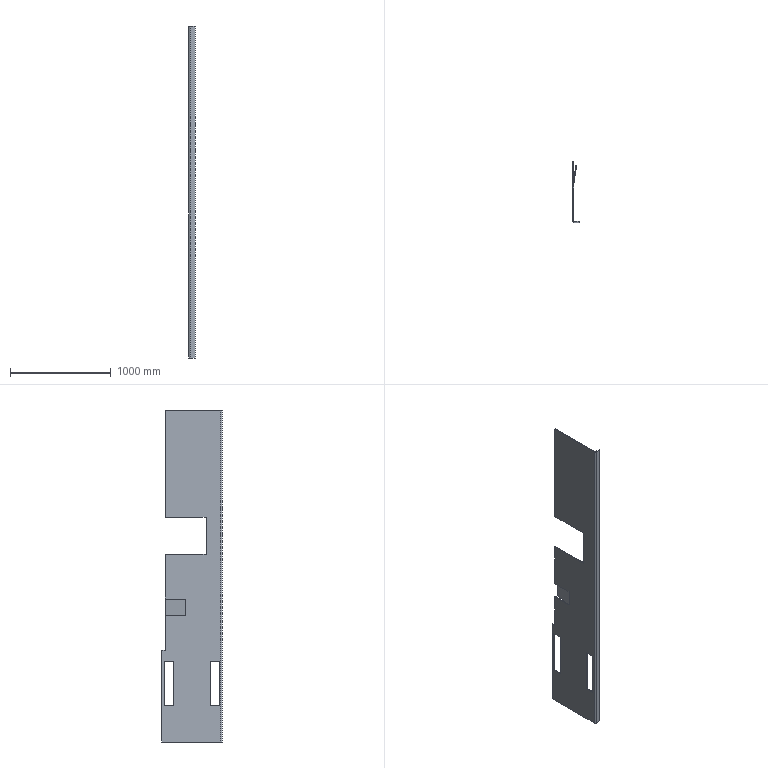Part | SolidWorks | features ICE 2, Extrusion 1, NetBlend 1 | 1 solid | 33 faces | box 65 x 605 x 3295 mm | volume 14782369 mm3 | plane 31 | cylinder 2 | commonest cylinder face diameters 16 x1 32 x1
STEP:
#1=CARTESIAN_POINT('',(0.,568.,909.));
#2=VERTEX_POINT('',#1);
#3=CARTESIAN_POINT('',(0.,568.,1259.));
#4=VERTEX_POINT('',#3);
#5=CARTESIAN_POINT('',(0.,568.,909.));
#6=DIRECTION('',(0.,0.,1.));
#7=VECTOR('',#6,1000.);
#8=LINE('',#5,#7);
#9=EDGE_CURVE('',#2,#4,#8,.T.);
#10=ORIENTED_EDGE('',*,*,#9,.T.);
#11=CARTESIAN_POINT('',(8.,568.,1259.));
#12=VERTEX_POINT('',#11);
#13=CARTESIAN_POINT('',(65.,568.,1259.));
#14=DIRECTION('',(-1.,0.,0.));
#15=VECTOR('',#14,1000.);
#16=LINE('',#13,#15);
#17=EDGE_CURVE('',#12,#4,#16,.T.);
#18=ORIENTED_EDGE('',*,*,#17,.F.);
#19=CARTESIAN_POINT('',(8.,568.,909.));
#20=VERTEX_POINT('',#19);
#21=CARTESIAN_POINT('',(8.,568.,3295.));
#22=DIRECTION('',(0.,0.,1.));
#23=VECTOR('',#22,1000.);
#24=LINE('',#21,#23);
#25=EDGE_CURVE('',#20,#12,#24,.T.);
#26=ORIENTED_EDGE('',*,*,#25,.F.);
#27=CARTESIAN_POINT('',(65.,568.,909.));
#28=DIRECTION('',(-1.,0.,0.));
#29=VECTOR('',#28,1000.);
#30=LINE('',#27,#29);
#31=EDGE_CURVE('',#20,#2,#30,.T.);
#32=ORIENTED_EDGE('',*,*,#31,.T.);
#33=EDGE_LOOP('',(#10,#18,#26,#32));
#34=FACE_OUTER_BOUND('',#33,.T.);
#35=CARTESIAN_POINT('',(65.,568.,909.));
#36=DIRECTION('',(0.,-1.,0.));
#37=DIRECTION('',(0.,0.,-1.));
#38=AXIS2_PLACEMENT_3D('',#35,#36,#37);
#39=PLANE('',#38);
#40=ADVANCED_FACE('',(#34),#39,.F.);
#41=CARTESIAN_POINT('',(8.,568.,1419.));
#42=VERTEX_POINT('',#41);
#43=CARTESIAN_POINT('',(8.,568.,1865.));
#44=VERTEX_POINT('',#43);
#45=CARTESIAN_POINT('',(8.,568.,3295.));
#46=DIRECTION('',(0.,0.,1.));
#47=VECTOR('',#46,1000.);
#48=LINE('',#45,#47);
#49=EDGE_CURVE('',#42,#44,#48,.T.);
#50=ORIENTED_EDGE('',*,*,#49,.F.);
#51=CARTESIAN_POINT('',(0.,568.,1419.));
#52=VERTEX_POINT('',#51);
#53=CARTESIAN_POINT('',(65.,568.,1419.));
#54=DIRECTION('',(-1.,0.,0.));
#55=VECTOR('',#54,1000.);
#56=LINE('',#53,#55);
#57=EDGE_CURVE('',#42,#52,#56,.T.);
#58=ORIENTED_EDGE('',*,*,#57,.T.);
#59=CARTESIAN_POINT('',(0.,568.,1865.));
#60=VERTEX_POINT('',#59);
#61=CARTESIAN_POINT('',(0.,568.,909.));
#62=DIRECTION('',(0.,0.,1.));
#63=VECTOR('',#62,1000.);
#64=LINE('',#61,#63);
#65=EDGE_CURVE('',#52,#60,#64,.T.);
#66=ORIENTED_EDGE('',*,*,#65,.T.);
#67=CARTESIAN_POINT('',(65.,568.,1865.));
#68=DIRECTION('',(1.,0.,0.));
#69=VECTOR('',#68,1000.);
#70=LINE('',#67,#69);
#71=EDGE_CURVE('',#60,#44,#70,.T.);
#72=ORIENTED_EDGE('',*,*,#71,.T.);
#73=EDGE_LOOP('',(#50,#58,#66,#72));
#74=FACE_OUTER_BOUND('',#73,.T.);
#75=CARTESIAN_POINT('',(65.,568.,909.));
#76=DIRECTION('',(0.,-1.,0.));
#77=DIRECTION('',(0.,0.,-1.));
#78=AXIS2_PLACEMENT_3D('',#75,#76,#77);
#79=PLANE('',#78);
#80=ADVANCED_FACE('',(#74),#79,.F.);
#81=CARTESIAN_POINT('',(0.,605.,909.));
#82=VERTEX_POINT('',#81);
#83=CARTESIAN_POINT('',(0.,605.,0.));
#84=VERTEX_POINT('',#83);
#85=CARTESIAN_POINT('',(0.,605.,3295.));
#86=DIRECTION('',(0.,0.,-1.));
#87=VECTOR('',#86,1000.);
#88=LINE('',#85,#87);
#89=EDGE_CURVE('',#82,#84,#88,.T.);
#90=ORIENTED_EDGE('',*,*,#89,.F.);
#91=CARTESIAN_POINT('',(8.,605.,909.));
#92=VERTEX_POINT('',#91);
#93=CARTESIAN_POINT('',(65.,605.,909.));
#94=DIRECTION('',(-1.,0.,0.));
#95=VECTOR('',#94,1000.);
#96=LINE('',#93,#95);
#97=EDGE_CURVE('',#92,#82,#96,.T.);
#98=ORIENTED_EDGE('',*,*,#97,.F.);
#99=CARTESIAN_POINT('',(8.,605.,0.));
#100=VERTEX_POINT('',#99);
#101=CARTESIAN_POINT('',(8.,605.,3295.));
#102=DIRECTION('',(0.,0.,-1.));
#103=VECTOR('',#102,1000.);
#104=LINE('',#101,#103);
#105=EDGE_CURVE('',#92,#100,#104,.T.);
#106=ORIENTED_EDGE('',*,*,#105,.T.);
#107=CARTESIAN_POINT('',(0.,605.,0.));
#108=DIRECTION('',(-1.,0.,0.));
#109=VECTOR('',#108,1000.);
#110=LINE('',#107,#109);
#111=EDGE_CURVE('',#100,#84,#110,.T.);
#112=ORIENTED_EDGE('',*,*,#111,.T.);
#113=EDGE_LOOP('',(#90,#98,#106,#112));
#114=FACE_OUTER_BOUND('',#113,.T.);
#115=CARTESIAN_POINT('',(0.,605.,3295.));
#116=DIRECTION('',(0.,-1.,0.));
#117=DIRECTION('',(0.,0.,-1.));
#118=AXIS2_PLACEMENT_3D('',#115,#116,#117);
#119=PLANE('',#118);
#120=ADVANCED_FACE('',(#114),#119,.F.);
#121=CARTESIAN_POINT('',(0.,580.,362.));
#122=VERTEX_POINT('',#121);
#123=CARTESIAN_POINT('',(0.,490.,362.));
#124=VERTEX_POINT('',#123);
#125=CARTESIAN_POINT('',(0.,580.,362.));
#126=DIRECTION('',(0.,-1.,0.));
#127=VECTOR('',#126,1000.);
#128=LINE('',#125,#127);
#129=EDGE_CURVE('',#122,#124,#128,.T.);
#130=ORIENTED_EDGE('',*,*,#129,.F.);
#131=CARTESIAN_POINT('',(0.,580.,802.));
#132=VERTEX_POINT('',#131);
#133=CARTESIAN_POINT('',(0.,580.,362.));
#134=DIRECTION('',(0.,0.,-1.));
#135=VECTOR('',#134,1000.);
#136=LINE('',#133,#135);
#137=EDGE_CURVE('',#132,#122,#136,.T.);
#138=ORIENTED_EDGE('',*,*,#137,.F.);
#139=CARTESIAN_POINT('',(0.,490.,802.));
#140=VERTEX_POINT('',#139);
#141=CARTESIAN_POINT('',(0.,580.,802.));
#142=DIRECTION('',(0.,1.,0.));
#143=VECTOR('',#142,1000.);
#144=LINE('',#141,#143);
#145=EDGE_CURVE('',#140,#132,#144,.T.);
#146=ORIENTED_EDGE('',*,*,#145,.F.);
#147=CARTESIAN_POINT('',(0.,490.,362.));
#148=DIRECTION('',(0.,0.,1.));
#149=VECTOR('',#148,1000.);
#150=LINE('',#147,#149);
#151=EDGE_CURVE('',#124,#140,#150,.T.);
#152=ORIENTED_EDGE('',*,*,#151,.F.);
#153=EDGE_LOOP('',(#130,#138,#146,#152));
#154=FACE_BOUND('',#153,.T.);
#155=CARTESIAN_POINT('',(0.,123.,802.));
#156=VERTEX_POINT('',#155);
#157=CARTESIAN_POINT('',(0.,123.,362.));
#158=VERTEX_POINT('',#157);
#159=CARTESIAN_POINT('',(0.,123.,362.));
#160=DIRECTION('',(0.,0.,-1.));
#161=VECTOR('',#160,1000.);
#162=LINE('',#159,#161);
#163=EDGE_CURVE('',#156,#158,#162,.T.);
#164=ORIENTED_EDGE('',*,*,#163,.F.);
#165=CARTESIAN_POINT('',(0.,33.,802.));
#166=VERTEX_POINT('',#165);
#167=CARTESIAN_POINT('',(0.,123.,802.));
#168=DIRECTION('',(0.,1.,0.));
#169=VECTOR('',#168,1000.);
#170=LINE('',#167,#169);
#171=EDGE_CURVE('',#166,#156,#170,.T.);
#172=ORIENTED_EDGE('',*,*,#171,.F.);
#173=CARTESIAN_POINT('',(0.,33.,362.));
#174=VERTEX_POINT('',#173);
#175=CARTESIAN_POINT('',(0.,33.,362.));
#176=DIRECTION('',(0.,0.,1.));
#177=VECTOR('',#176,1000.);
#178=LINE('',#175,#177);
#179=EDGE_CURVE('',#174,#166,#178,.T.);
#180=ORIENTED_EDGE('',*,*,#179,.F.);
#181=CARTESIAN_POINT('',(0.,123.,362.));
#182=DIRECTION('',(0.,-1.,0.));
#183=VECTOR('',#182,1000.);
#184=LINE('',#181,#183);
#185=EDGE_CURVE('',#158,#174,#184,.T.);
#186=ORIENTED_EDGE('',*,*,#185,.F.);
#187=EDGE_LOOP('',(#164,#172,#180,#186));
#188=FACE_BOUND('',#187,.T.);
#189=CARTESIAN_POINT('',(0.,368.,1259.));
#190=VERTEX_POINT('',#189);
#191=CARTESIAN_POINT('',(0.,368.,1419.));
#192=VERTEX_POINT('',#191);
#193=CARTESIAN_POINT('',(0.,368.,1259.));
#194=DIRECTION('',(0.,0.,1.));
#195=VECTOR('',#194,1000.);
#196=LINE('',#193,#195);
#197=EDGE_CURVE('',#190,#192,#196,.T.);
#198=ORIENTED_EDGE('',*,*,#197,.F.);
#199=CARTESIAN_POINT('',(0.,568.,1259.));
#200=DIRECTION('',(0.,-1.,0.));
#201=VECTOR('',#200,1000.);
#202=LINE('',#199,#201);
#203=EDGE_CURVE('',#4,#190,#202,.T.);
#204=ORIENTED_EDGE('',*,*,#203,.F.);
#205=ORIENTED_EDGE('',*,*,#9,.F.);
#206=CARTESIAN_POINT('',(0.,605.,909.));
#207=DIRECTION('',(0.,-1.,0.));
#208=VECTOR('',#207,1000.);
#209=LINE('',#206,#208);
#210=EDGE_CURVE('',#82,#2,#209,.T.);
#211=ORIENTED_EDGE('',*,*,#210,.F.);
#212=ORIENTED_EDGE('',*,*,#89,.T.);
#213=CARTESIAN_POINT('',(0.,16.,0.));
#214=VERTEX_POINT('',#213);
#215=CARTESIAN_POINT('',(0.,16.,0.));
#216=DIRECTION('',(0.,-1.,0.));
#217=VECTOR('',#216,1000.);
#218=LINE('',#215,#217);
#219=EDGE_CURVE('',#84,#214,#218,.T.);
#220=ORIENTED_EDGE('',*,*,#219,.T.);
#221=CARTESIAN_POINT('',(0.,16.,3295.));
#222=VERTEX_POINT('',#221);
#223=CARTESIAN_POINT('',(0.,16.,3295.));
#224=DIRECTION('',(0.,0.,-1.));
#225=VECTOR('',#224,1000.);
#226=LINE('',#223,#225);
#227=EDGE_CURVE('',#222,#214,#226,.T.);
#228=ORIENTED_EDGE('',*,*,#227,.F.);
#229=CARTESIAN_POINT('',(0.,568.,3295.));
#230=VERTEX_POINT('',#229);
#231=CARTESIAN_POINT('',(0.,16.,3295.));
#232=DIRECTION('',(0.,-1.,0.));
#233=VECTOR('',#232,1000.);
#234=LINE('',#231,#233);
#235=EDGE_CURVE('',#230,#222,#234,.T.);
#236=ORIENTED_EDGE('',*,*,#235,.F.);
#237=CARTESIAN_POINT('',(0.,568.,2233.));
#238=VERTEX_POINT('',#237);
#239=CARTESIAN_POINT('',(0.,568.,909.));
#240=DIRECTION('',(0.,0.,1.));
#241=VECTOR('',#240,1000.);
#242=LINE('',#239,#241);
#243=EDGE_CURVE('',#238,#230,#242,.T.);
#244=ORIENTED_EDGE('',*,*,#243,.F.);
#245=CARTESIAN_POINT('',(0.,163.,2233.));
#246=VERTEX_POINT('',#245);
#247=CARTESIAN_POINT('',(0.,568.,2233.));
#248=DIRECTION('',(0.,1.,0.));
#249=VECTOR('',#248,1000.);
#250=LINE('',#247,#249);
#251=EDGE_CURVE('',#246,#238,#250,.T.);
#252=ORIENTED_EDGE('',*,*,#251,.F.);
#253=CARTESIAN_POINT('',(0.,163.,1865.));
#254=VERTEX_POINT('',#253);
#255=CARTESIAN_POINT('',(0.,163.,1865.));
#256=DIRECTION('',(0.,0.,1.));
#257=VECTOR('',#256,1000.);
#258=LINE('',#255,#257);
#259=EDGE_CURVE('',#254,#246,#258,.T.);
#260=ORIENTED_EDGE('',*,*,#259,.F.);
#261=CARTESIAN_POINT('',(0.,568.,1865.));
#262=DIRECTION('',(0.,-1.,0.));
#263=VECTOR('',#262,1000.);
#264=LINE('',#261,#263);
#265=EDGE_CURVE('',#60,#254,#264,.T.);
#266=ORIENTED_EDGE('',*,*,#265,.F.);
#267=ORIENTED_EDGE('',*,*,#65,.F.);
#268=CARTESIAN_POINT('',(0.,368.,1419.));
#269=DIRECTION('',(0.,1.,0.));
#270=VECTOR('',#269,1000.);
#271=LINE('',#268,#270);
#272=EDGE_CURVE('',#192,#52,#271,.T.);
#273=ORIENTED_EDGE('',*,*,#272,.F.);
#274=EDGE_LOOP('',(#198,#204,#205,#211,#212,#220,#228,#236,#244,#252,#260,#266,#267,#273));
#275=FACE_OUTER_BOUND('',#274,.T.);
#276=CARTESIAN_POINT('',(0.,16.,3295.));
#277=DIRECTION('',(1.,0.,0.));
#278=DIRECTION('',(0.,0.,-1.));
#279=AXIS2_PLACEMENT_3D('',#276,#277,#278);
#280=PLANE('',#279);
#281=ADVANCED_FACE('',(#154,#188,#275),#280,.F.);
#282=CARTESIAN_POINT('',(16.,0.,0.));
#283=VERTEX_POINT('',#282);
#284=CARTESIAN_POINT('',(16.,16.,0.));
#285=DIRECTION('',(0.,0.,1.));
#286=DIRECTION('',(1.,0.,0.));
#287=AXIS2_PLACEMENT_3D('',#284,#285,#286);
#288=CIRCLE('',#287,16.);
#289=EDGE_CURVE('',#214,#283,#288,.T.);
#290=ORIENTED_EDGE('',*,*,#289,.T.);
#291=CARTESIAN_POINT('',(16.,0.,3295.));
#292=VERTEX_POINT('',#291);
#293=CARTESIAN_POINT('',(16.,0.,3295.));
#294=DIRECTION('',(0.,0.,-1.));
#295=VECTOR('',#294,1000.);
#296=LINE('',#293,#295);
#297=EDGE_CURVE('',#292,#283,#296,.T.);
#298=ORIENTED_EDGE('',*,*,#297,.F.);
#299=CARTESIAN_POINT('',(16.,16.,3295.));
#300=DIRECTION('',(0.,0.,1.));
#301=DIRECTION('',(1.,0.,0.));
#302=AXIS2_PLACEMENT_3D('',#299,#300,#301);
#303=CIRCLE('',#302,16.);
#304=EDGE_CURVE('',#222,#292,#303,.T.);
#305=ORIENTED_EDGE('',*,*,#304,.F.);
#306=ORIENTED_EDGE('',*,*,#227,.T.);
#307=EDGE_LOOP('',(#290,#298,#305,#306));
#308=FACE_OUTER_BOUND('',#307,.T.);
#309=CARTESIAN_POINT('',(16.,16.,3295.));
#310=DIRECTION('',(0.,0.,-1.));
#311=DIRECTION('',(-1.,0.,0.));
#312=AXIS2_PLACEMENT_3D('',#309,#310,#311);
#313=CYLINDRICAL_SURFACE('',#312,16.);
#314=ADVANCED_FACE('',(#308),#313,.T.);
#315=CARTESIAN_POINT('',(65.,0.,0.));
#316=VERTEX_POINT('',#315);
#317=CARTESIAN_POINT('',(65.,0.,0.));
#318=DIRECTION('',(1.,0.,0.));
#319=VECTOR('',#318,1000.);
#320=LINE('',#317,#319);
#321=EDGE_CURVE('',#283,#316,#320,.T.);
#322=ORIENTED_EDGE('',*,*,#321,.T.);
#323=CARTESIAN_POINT('',(65.,0.,3295.));
#324=VERTEX_POINT('',#323);
#325=CARTESIAN_POINT('',(65.,0.,3295.));
#326=DIRECTION('',(0.,0.,-1.));
#327=VECTOR('',#326,1000.);
#328=LINE('',#325,#327);
#329=EDGE_CURVE('',#324,#316,#328,.T.);
#330=ORIENTED_EDGE('',*,*,#329,.F.);
#331=CARTESIAN_POINT('',(65.,0.,3295.));
#332=DIRECTION('',(1.,0.,0.));
#333=VECTOR('',#332,1000.);
#334=LINE('',#331,#333);
#335=EDGE_CURVE('',#292,#324,#334,.T.);
#336=ORIENTED_EDGE('',*,*,#335,.F.);
#337=ORIENTED_EDGE('',*,*,#297,.T.);
#338=EDGE_LOOP('',(#322,#330,#336,#337));
#339=FACE_OUTER_BOUND('',#338,.T.);
#340=CARTESIAN_POINT('',(65.,0.,3295.));
#341=DIRECTION('',(0.,1.,0.));
#342=DIRECTION('',(-1.,0.,0.));
#343=AXIS2_PLACEMENT_3D('',#340,#341,#342);
#344=PLANE('',#343);
#345=ADVANCED_FACE('',(#339),#344,.F.);
#346=CARTESIAN_POINT('',(65.,8.,0.));
#347=VERTEX_POINT('',#346);
#348=CARTESIAN_POINT('',(65.,8.,0.));
#349=DIRECTION('',(0.,1.,0.));
#350=VECTOR('',#349,1000.);
#351=LINE('',#348,#350);
#352=EDGE_CURVE('',#316,#347,#351,.T.);
#353=ORIENTED_EDGE('',*,*,#352,.T.);
#354=CARTESIAN_POINT('',(65.,8.,3295.));
#355=VERTEX_POINT('',#354);
#356=CARTESIAN_POINT('',(65.,8.,3295.));
#357=DIRECTION('',(0.,0.,-1.));
#358=VECTOR('',#357,1000.);
#359=LINE('',#356,#358);
#360=EDGE_CURVE('',#355,#347,#359,.T.);
#361=ORIENTED_EDGE('',*,*,#360,.F.);
#362=CARTESIAN_POINT('',(65.,8.,3295.));
#363=DIRECTION('',(0.,1.,0.));
#364=VECTOR('',#363,1000.);
#365=LINE('',#362,#364);
#366=EDGE_CURVE('',#324,#355,#365,.T.);
#367=ORIENTED_EDGE('',*,*,#366,.F.);
#368=ORIENTED_EDGE('',*,*,#329,.T.);
#369=EDGE_LOOP('',(#353,#361,#367,#368));
#370=FACE_OUTER_BOUND('',#369,.T.);
#371=CARTESIAN_POINT('',(65.,8.,3295.));
#372=DIRECTION('',(-1.,0.,0.));
#373=DIRECTION('',(0.,0.,1.));
#374=AXIS2_PLACEMENT_3D('',#371,#372,#373);
#375=PLANE('',#374);
#376=ADVANCED_FACE('',(#370),#375,.F.);
#377=CARTESIAN_POINT('',(16.,8.,0.));
#378=VERTEX_POINT('',#377);
#379=CARTESIAN_POINT('',(16.,8.,0.));
#380=DIRECTION('',(-1.,0.,0.));
#381=VECTOR('',#380,1000.);
#382=LINE('',#379,#381);
#383=EDGE_CURVE('',#347,#378,#382,.T.);
#384=ORIENTED_EDGE('',*,*,#383,.T.);
#385=CARTESIAN_POINT('',(16.,8.,3295.));
#386=VERTEX_POINT('',#385);
#387=CARTESIAN_POINT('',(16.,8.,3295.));
#388=DIRECTION('',(0.,0.,-1.));
#389=VECTOR('',#388,1000.);
#390=LINE('',#387,#389);
#391=EDGE_CURVE('',#386,#378,#390,.T.);
#392=ORIENTED_EDGE('',*,*,#391,.F.);
#393=CARTESIAN_POINT('',(16.,8.,3295.));
#394=DIRECTION('',(-1.,0.,0.));
#395=VECTOR('',#394,1000.);
#396=LINE('',#393,#395);
#397=EDGE_CURVE('',#355,#386,#396,.T.);
#398=ORIENTED_EDGE('',*,*,#397,.F.);
#399=ORIENTED_EDGE('',*,*,#360,.T.);
#400=EDGE_LOOP('',(#384,#392,#398,#399));
#401=FACE_OUTER_BOUND('',#400,.T.);
#402=CARTESIAN_POINT('',(16.,8.,3295.));
#403=DIRECTION('',(0.,-1.,0.));
#404=DIRECTION('',(0.,0.,-1.));
#405=AXIS2_PLACEMENT_3D('',#402,#403,#404);
#406=PLANE('',#405);
#407=ADVANCED_FACE('',(#401),#406,.F.);
#408=CARTESIAN_POINT('',(8.,16.,0.));
#409=VERTEX_POINT('',#408);
#410=CARTESIAN_POINT('',(16.,16.,0.));
#411=DIRECTION('',(0.,0.,-1.));
#412=DIRECTION('',(1.,0.,0.));
#413=AXIS2_PLACEMENT_3D('',#410,#411,#412);
#414=CIRCLE('',#413,8.);
#415=EDGE_CURVE('',#378,#409,#414,.T.);
#416=ORIENTED_EDGE('',*,*,#415,.T.);
#417=CARTESIAN_POINT('',(8.,16.,3295.));
#418=VERTEX_POINT('',#417);
#419=CARTESIAN_POINT('',(8.,16.,3295.));
#420=DIRECTION('',(0.,0.,-1.));
#421=VECTOR('',#420,1000.);
#422=LINE('',#419,#421);
#423=EDGE_CURVE('',#418,#409,#422,.T.);
#424=ORIENTED_EDGE('',*,*,#423,.F.);
#425=CARTESIAN_POINT('',(16.,16.,3295.));
#426=DIRECTION('',(0.,0.,-1.));
#427=DIRECTION('',(1.,0.,0.));
#428=AXIS2_PLACEMENT_3D('',#425,#426,#427);
#429=CIRCLE('',#428,8.);
#430=EDGE_CURVE('',#386,#418,#429,.T.);
#431=ORIENTED_EDGE('',*,*,#430,.F.);
#432=ORIENTED_EDGE('',*,*,#391,.T.);
#433=EDGE_LOOP('',(#416,#424,#431,#432));
#434=FACE_OUTER_BOUND('',#433,.T.);
#435=CARTESIAN_POINT('',(16.,16.,3295.));
#436=DIRECTION('',(0.,0.,-1.));
#437=DIRECTION('',(-1.,0.,0.));
#438=AXIS2_PLACEMENT_3D('',#435,#436,#437);
#439=CYLINDRICAL_SURFACE('',#438,8.);
#440=ADVANCED_FACE('',(#434),#439,.F.);
#441=CARTESIAN_POINT('',(8.,490.,802.));
#442=VERTEX_POINT('',#441);
#443=CARTESIAN_POINT('',(8.,580.,802.));
#444=VERTEX_POINT('',#443);
#445=CARTESIAN_POINT('',(8.,605.,802.));
#446=DIRECTION('',(0.,1.,0.));
#447=VECTOR('',#446,1000.);
#448=LINE('',#445,#447);
#449=EDGE_CURVE('',#442,#444,#448,.T.);
#450=ORIENTED_EDGE('',*,*,#449,.T.);
#451=CARTESIAN_POINT('',(8.,580.,362.));
#452=VERTEX_POINT('',#451);
#453=CARTESIAN_POINT('',(8.,580.,3295.));
#454=DIRECTION('',(0.,0.,-1.));
#455=VECTOR('',#454,1000.);
#456=LINE('',#453,#455);
#457=EDGE_CURVE('',#444,#452,#456,.T.);
#458=ORIENTED_EDGE('',*,*,#457,.T.);
#459=CARTESIAN_POINT('',(8.,490.,362.));
#460=VERTEX_POINT('',#459);
#461=CARTESIAN_POINT('',(8.,605.,362.));
#462=DIRECTION('',(0.,-1.,0.));
#463=VECTOR('',#462,1000.);
#464=LINE('',#461,#463);
#465=EDGE_CURVE('',#452,#460,#464,.T.);
#466=ORIENTED_EDGE('',*,*,#465,.T.);
#467=CARTESIAN_POINT('',(8.,490.,3295.));
#468=DIRECTION('',(0.,0.,1.));
#469=VECTOR('',#468,1000.);
#470=LINE('',#467,#469);
#471=EDGE_CURVE('',#460,#442,#470,.T.);
#472=ORIENTED_EDGE('',*,*,#471,.T.);
#473=EDGE_LOOP('',(#450,#458,#466,#472));
#474=FACE_BOUND('',#473,.T.);
#475=CARTESIAN_POINT('',(8.,33.,362.));
#476=VERTEX_POINT('',#475);
#477=CARTESIAN_POINT('',(8.,33.,802.));
#478=VERTEX_POINT('',#477);
#479=CARTESIAN_POINT('',(8.,33.,3295.));
#480=DIRECTION('',(0.,0.,1.));
#481=VECTOR('',#480,1000.);
#482=LINE('',#479,#481);
#483=EDGE_CURVE('',#476,#478,#482,.T.);
#484=ORIENTED_EDGE('',*,*,#483,.T.);
#485=CARTESIAN_POINT('',(8.,123.,802.));
#486=VERTEX_POINT('',#485);
#487=CARTESIAN_POINT('',(8.,605.,802.));
#488=DIRECTION('',(0.,1.,0.));
#489=VECTOR('',#488,1000.);
#490=LINE('',#487,#489);
#491=EDGE_CURVE('',#478,#486,#490,.T.);
#492=ORIENTED_EDGE('',*,*,#491,.T.);
#493=CARTESIAN_POINT('',(8.,123.,362.));
#494=VERTEX_POINT('',#493);
#495=CARTESIAN_POINT('',(8.,123.,3295.));
#496=DIRECTION('',(0.,0.,-1.));
#497=VECTOR('',#496,1000.);
#498=LINE('',#495,#497);
#499=EDGE_CURVE('',#486,#494,#498,.T.);
#500=ORIENTED_EDGE('',*,*,#499,.T.);
#501=CARTESIAN_POINT('',(8.,605.,362.));
#502=DIRECTION('',(0.,-1.,0.));
#503=VECTOR('',#502,1000.);
#504=LINE('',#501,#503);
#505=EDGE_CURVE('',#494,#476,#504,.T.);
#506=ORIENTED_EDGE('',*,*,#505,.T.);
#507=EDGE_LOOP('',(#484,#492,#500,#506));
#508=FACE_BOUND('',#507,.T.);
#509=CARTESIAN_POINT('',(8.,418.51,1259.));
#510=VERTEX_POINT('',#509);
#511=CARTESIAN_POINT('',(8.,367.985,1259.));
#512=VERTEX_POINT('',#511);
#513=CARTESIAN_POINT('',(8.,605.,1259.));
#514=DIRECTION('',(0.,-1.,0.));
#515=VECTOR('',#514,1000.);
#516=LINE('',#513,#515);
#517=EDGE_CURVE('',#510,#512,#516,.T.);
#518=ORIENTED_EDGE('',*,*,#517,.T.);
#519=CARTESIAN_POINT('',(8.,367.985,1419.));
#520=VERTEX_POINT('',#519);
#521=CARTESIAN_POINT('',(8.,367.985,3295.));
#522=DIRECTION('',(0.,0.,1.));
#523=VECTOR('',#522,1000.);
#524=LINE('',#521,#523);
#525=EDGE_CURVE('',#512,#520,#524,.T.);
#526=ORIENTED_EDGE('',*,*,#525,.T.);
#527=CARTESIAN_POINT('',(8.,418.51,1419.));
#528=VERTEX_POINT('',#527);
#529=CARTESIAN_POINT('',(8.,605.,1419.));
#530=DIRECTION('',(0.,1.,0.));
#531=VECTOR('',#530,1000.);
#532=LINE('',#529,#531);
#533=EDGE_CURVE('',#520,#528,#532,.T.);
#534=ORIENTED_EDGE('',*,*,#533,.T.);
#535=CARTESIAN_POINT('',(8.,605.,1419.));
#536=DIRECTION('',(0.,1.,0.));
#537=VECTOR('',#536,1000.);
#538=LINE('',#535,#537);
#539=EDGE_CURVE('',#528,#42,#538,.T.);
#540=ORIENTED_EDGE('',*,*,#539,.T.);
#541=ORIENTED_EDGE('',*,*,#49,.T.);
#542=CARTESIAN_POINT('',(8.,163.,1865.));
#543=VERTEX_POINT('',#542);
#544=CARTESIAN_POINT('',(8.,605.,1865.));
#545=DIRECTION('',(0.,-1.,0.));
#546=VECTOR('',#545,1000.);
#547=LINE('',#544,#546);
#548=EDGE_CURVE('',#44,#543,#547,.T.);
#549=ORIENTED_EDGE('',*,*,#548,.T.);
#550=CARTESIAN_POINT('',(8.,163.,2233.));
#551=VERTEX_POINT('',#550);
#552=CARTESIAN_POINT('',(8.,163.,3295.));
#553=DIRECTION('',(0.,0.,1.));
#554=VECTOR('',#553,1000.);
#555=LINE('',#552,#554);
#556=EDGE_CURVE('',#543,#551,#555,.T.);
#557=ORIENTED_EDGE('',*,*,#556,.T.);
#558=CARTESIAN_POINT('',(8.,568.,2233.));
#559=VERTEX_POINT('',#558);
#560=CARTESIAN_POINT('',(8.,605.,2233.));
#561=DIRECTION('',(0.,1.,0.));
#562=VECTOR('',#561,1000.);
#563=LINE('',#560,#562);
#564=EDGE_CURVE('',#551,#559,#563,.T.);
#565=ORIENTED_EDGE('',*,*,#564,.T.);
#566=CARTESIAN_POINT('',(8.,568.,3295.));
#567=VERTEX_POINT('',#566);
#568=CARTESIAN_POINT('',(8.,568.,3295.));
#569=DIRECTION('',(0.,0.,1.));
#570=VECTOR('',#569,1000.);
#571=LINE('',#568,#570);
#572=EDGE_CURVE('',#559,#567,#571,.T.);
#573=ORIENTED_EDGE('',*,*,#572,.T.);
#574=CARTESIAN_POINT('',(8.,605.,3295.));
#575=DIRECTION('',(0.,1.,0.));
#576=VECTOR('',#575,1000.);
#577=LINE('',#574,#576);
#578=EDGE_CURVE('',#418,#567,#577,.T.);
#579=ORIENTED_EDGE('',*,*,#578,.F.);
#580=ORIENTED_EDGE('',*,*,#423,.T.);
#581=CARTESIAN_POINT('',(8.,605.,0.));
#582=DIRECTION('',(0.,1.,0.));
#583=VECTOR('',#582,1000.);
#584=LINE('',#581,#583);
#585=EDGE_CURVE('',#409,#100,#584,.T.);
#586=ORIENTED_EDGE('',*,*,#585,.T.);
#587=ORIENTED_EDGE('',*,*,#105,.F.);
#588=CARTESIAN_POINT('',(8.,605.,909.));
#589=DIRECTION('',(0.,-1.,0.));
#590=VECTOR('',#589,1000.);
#591=LINE('',#588,#590);
#592=EDGE_CURVE('',#92,#20,#591,.T.);
#593=ORIENTED_EDGE('',*,*,#592,.T.);
#594=ORIENTED_EDGE('',*,*,#25,.T.);
#595=CARTESIAN_POINT('',(8.,605.,1259.));
#596=DIRECTION('',(0.,-1.,0.));
#597=VECTOR('',#596,1000.);
#598=LINE('',#595,#597);
#599=EDGE_CURVE('',#12,#510,#598,.T.);
#600=ORIENTED_EDGE('',*,*,#599,.T.);
#601=EDGE_LOOP('',(#518,#526,#534,#540,#541,#549,#557,#565,#573,#579,#580,#586,#587,#593,#594,#600));
#602=FACE_OUTER_BOUND('',#601,.T.);
#603=CARTESIAN_POINT('',(8.,605.,3295.));
#604=DIRECTION('',(-1.,0.,0.));
#605=DIRECTION('',(0.,-1.,0.));
#606=AXIS2_PLACEMENT_3D('',#603,#604,#605);
#607=PLANE('',#606);
#608=ADVANCED_FACE('',(#474,#508,#602),#607,.F.);
#609=CARTESIAN_POINT('',(16.,568.,3295.));
#610=DIRECTION('',(1.,0.,0.));
#611=VECTOR('',#610,1000.);
#612=LINE('',#609,#611);
#613=EDGE_CURVE('',#230,#567,#612,.T.);
#614=ORIENTED_EDGE('',*,*,#613,.F.);
#615=ORIENTED_EDGE('',*,*,#235,.T.);
#616=ORIENTED_EDGE('',*,*,#304,.T.);
#617=ORIENTED_EDGE('',*,*,#335,.T.);
#618=ORIENTED_EDGE('',*,*,#366,.T.);
#619=ORIENTED_EDGE('',*,*,#397,.T.);
#620=ORIENTED_EDGE('',*,*,#430,.T.);
#621=ORIENTED_EDGE('',*,*,#578,.T.);
#622=EDGE_LOOP('',(#614,#615,#616,#617,#618,#619,#620,#621));
#623=FACE_OUTER_BOUND('',#622,.T.);
#624=CARTESIAN_POINT('',(16.,16.,3295.));
#625=DIRECTION('',(0.,0.,1.));
#626=DIRECTION('',(1.,0.,0.));
#627=AXIS2_PLACEMENT_3D('',#624,#625,#626);
#628=PLANE('',#627);
#629=ADVANCED_FACE('',(#623),#628,.T.);
#630=ORIENTED_EDGE('',*,*,#111,.F.);
#631=ORIENTED_EDGE('',*,*,#585,.F.);
#632=ORIENTED_EDGE('',*,*,#415,.F.);
#633=ORIENTED_EDGE('',*,*,#383,.F.);
#634=ORIENTED_EDGE('',*,*,#352,.F.);
#635=ORIENTED_EDGE('',*,*,#321,.F.);
#636=ORIENTED_EDGE('',*,*,#289,.F.);
#637=ORIENTED_EDGE('',*,*,#219,.F.);
#638=EDGE_LOOP('',(#630,#631,#632,#633,#634,#635,#636,#637));
#639=FACE_OUTER_BOUND('',#638,.T.);
#640=CARTESIAN_POINT('',(16.,16.,0.));
#641=DIRECTION('',(0.,0.,1.));
#642=DIRECTION('',(1.,0.,0.));
#643=AXIS2_PLACEMENT_3D('',#640,#641,#642);
#644=PLANE('',#643);
#645=ADVANCED_FACE('',(#639),#644,.F.);
#646=ORIENTED_EDGE('',*,*,#97,.T.);
#647=ORIENTED_EDGE('',*,*,#210,.T.);
#648=ORIENTED_EDGE('',*,*,#31,.F.);
#649=ORIENTED_EDGE('',*,*,#592,.F.);
#650=EDGE_LOOP('',(#646,#647,#648,#649));
#651=FACE_OUTER_BOUND('',#650,.T.);
#652=CARTESIAN_POINT('',(65.,605.,909.));
#653=DIRECTION('',(0.,0.,-1.));
#654=DIRECTION('',(-1.,0.,0.));
#655=AXIS2_PLACEMENT_3D('',#652,#653,#654);
#656=PLANE('',#655);
#657=ADVANCED_FACE('',(#651),#656,.F.);
#658=ORIENTED_EDGE('',*,*,#572,.F.);
#659=CARTESIAN_POINT('',(65.,568.,2233.));
#660=DIRECTION('',(-1.,0.,0.));
#661=VECTOR('',#660,1000.);
#662=LINE('',#659,#661);
#663=EDGE_CURVE('',#559,#238,#662,.T.);
#664=ORIENTED_EDGE('',*,*,#663,.T.);
#665=ORIENTED_EDGE('',*,*,#243,.T.);
#666=ORIENTED_EDGE('',*,*,#613,.T.);
#667=EDGE_LOOP('',(#658,#664,#665,#666));
#668=FACE_OUTER_BOUND('',#667,.T.);
#669=CARTESIAN_POINT('',(65.,568.,909.));
#670=DIRECTION('',(0.,-1.,0.));
#671=DIRECTION('',(0.,0.,-1.));
#672=AXIS2_PLACEMENT_3D('',#669,#670,#671);
#673=PLANE('',#672);
#674=ADVANCED_FACE('',(#668),#673,.F.);
#675=CARTESIAN_POINT('',(65.,33.,802.));
#676=DIRECTION('',(-1.,0.,0.));
#677=VECTOR('',#676,1000.);
#678=LINE('',#675,#677);
#679=EDGE_CURVE('',#478,#166,#678,.T.);
#680=ORIENTED_EDGE('',*,*,#679,.T.);
#681=ORIENTED_EDGE('',*,*,#171,.T.);
#682=CARTESIAN_POINT('',(65.,123.,802.));
#683=DIRECTION('',(-1.,0.,0.));
#684=VECTOR('',#683,1000.);
#685=LINE('',#682,#684);
#686=EDGE_CURVE('',#486,#156,#685,.T.);
#687=ORIENTED_EDGE('',*,*,#686,.F.);
#688=ORIENTED_EDGE('',*,*,#491,.F.);
#689=EDGE_LOOP('',(#680,#681,#687,#688));
#690=FACE_OUTER_BOUND('',#689,.T.);
#691=CARTESIAN_POINT('',(65.,123.,802.));
#692=DIRECTION('',(0.,0.,1.));
#693=DIRECTION('',(1.,0.,0.));
#694=AXIS2_PLACEMENT_3D('',#691,#692,#693);
#695=PLANE('',#694);
#696=ADVANCED_FACE('',(#690),#695,.F.);
#697=CARTESIAN_POINT('',(65.,33.,362.));
#698=DIRECTION('',(-1.,0.,0.));
#699=VECTOR('',#698,1000.);
#700=LINE('',#697,#699);
#701=EDGE_CURVE('',#476,#174,#700,.T.);
#702=ORIENTED_EDGE('',*,*,#701,.T.);
#703=ORIENTED_EDGE('',*,*,#179,.T.);
#704=ORIENTED_EDGE('',*,*,#679,.F.);
#705=ORIENTED_EDGE('',*,*,#483,.F.);
#706=EDGE_LOOP('',(#702,#703,#704,#705));
#707=FACE_OUTER_BOUND('',#706,.T.);
#708=CARTESIAN_POINT('',(65.,33.,362.));
#709=DIRECTION('',(0.,-1.,0.));
#710=DIRECTION('',(0.,0.,-1.));
#711=AXIS2_PLACEMENT_3D('',#708,#709,#710);
#712=PLANE('',#711);
#713=ADVANCED_FACE('',(#707),#712,.F.);
#714=CARTESIAN_POINT('',(65.,123.,362.));
#715=DIRECTION('',(-1.,0.,0.));
#716=VECTOR('',#715,1000.);
#717=LINE('',#714,#716);
#718=EDGE_CURVE('',#494,#158,#717,.T.);
#719=ORIENTED_EDGE('',*,*,#718,.T.);
#720=ORIENTED_EDGE('',*,*,#185,.T.);
#721=ORIENTED_EDGE('',*,*,#701,.F.);
#722=ORIENTED_EDGE('',*,*,#505,.F.);
#723=EDGE_LOOP('',(#719,#720,#721,#722));
#724=FACE_OUTER_BOUND('',#723,.T.);
#725=CARTESIAN_POINT('',(65.,123.,362.));
#726=DIRECTION('',(0.,0.,-1.));
#727=DIRECTION('',(-1.,0.,0.));
#728=AXIS2_PLACEMENT_3D('',#725,#726,#727);
#729=PLANE('',#728);
#730=ADVANCED_FACE('',(#724),#729,.F.);
#731=ORIENTED_EDGE('',*,*,#686,.T.);
#732=ORIENTED_EDGE('',*,*,#163,.T.);
#733=ORIENTED_EDGE('',*,*,#718,.F.);
#734=ORIENTED_EDGE('',*,*,#499,.F.);
#735=EDGE_LOOP('',(#731,#732,#733,#734));
#736=FACE_OUTER_BOUND('',#735,.T.);
#737=CARTESIAN_POINT('',(65.,123.,362.));
#738=DIRECTION('',(0.,1.,0.));
#739=DIRECTION('',(0.,0.,1.));
#740=AXIS2_PLACEMENT_3D('',#737,#738,#739);
#741=PLANE('',#740);
#742=ADVANCED_FACE('',(#736),#741,.F.);
#743=CARTESIAN_POINT('',(65.,580.,802.));
#744=DIRECTION('',(-1.,0.,0.));
#745=VECTOR('',#744,1000.);
#746=LINE('',#743,#745);
#747=EDGE_CURVE('',#444,#132,#746,.T.);
#748=ORIENTED_EDGE('',*,*,#747,.T.);
#749=ORIENTED_EDGE('',*,*,#137,.T.);
#750=CARTESIAN_POINT('',(65.,580.,362.));
#751=DIRECTION('',(-1.,0.,0.));
#752=VECTOR('',#751,1000.);
#753=LINE('',#750,#752);
#754=EDGE_CURVE('',#452,#122,#753,.T.);
#755=ORIENTED_EDGE('',*,*,#754,.F.);
#756=ORIENTED_EDGE('',*,*,#457,.F.);
#757=EDGE_LOOP('',(#748,#749,#755,#756));
#758=FACE_OUTER_BOUND('',#757,.T.);
#759=CARTESIAN_POINT('',(65.,580.,362.));
#760=DIRECTION('',(0.,1.,0.));
#761=DIRECTION('',(0.,0.,1.));
#762=AXIS2_PLACEMENT_3D('',#759,#760,#761);
#763=PLANE('',#762);
#764=ADVANCED_FACE('',(#758),#763,.F.);
#765=CARTESIAN_POINT('',(65.,490.,802.));
#766=DIRECTION('',(-1.,0.,0.));
#767=VECTOR('',#766,1000.);
#768=LINE('',#765,#767);
#769=EDGE_CURVE('',#442,#140,#768,.T.);
#770=ORIENTED_EDGE('',*,*,#769,.T.);
#771=ORIENTED_EDGE('',*,*,#145,.T.);
#772=ORIENTED_EDGE('',*,*,#747,.F.);
#773=ORIENTED_EDGE('',*,*,#449,.F.);
#774=EDGE_LOOP('',(#770,#771,#772,#773));
#775=FACE_OUTER_BOUND('',#774,.T.);
#776=CARTESIAN_POINT('',(65.,580.,802.));
#777=DIRECTION('',(0.,0.,1.));
#778=DIRECTION('',(0.,-1.,0.));
#779=AXIS2_PLACEMENT_3D('',#776,#777,#778);
#780=PLANE('',#779);
#781=ADVANCED_FACE('',(#775),#780,.F.);
#782=CARTESIAN_POINT('',(65.,490.,362.));
#783=DIRECTION('',(-1.,0.,0.));
#784=VECTOR('',#783,1000.);
#785=LINE('',#782,#784);
#786=EDGE_CURVE('',#460,#124,#785,.T.);
#787=ORIENTED_EDGE('',*,*,#786,.T.);
#788=ORIENTED_EDGE('',*,*,#151,.T.);
#789=ORIENTED_EDGE('',*,*,#769,.F.);
#790=ORIENTED_EDGE('',*,*,#471,.F.);
#791=EDGE_LOOP('',(#787,#788,#789,#790));
#792=FACE_OUTER_BOUND('',#791,.T.);
#793=CARTESIAN_POINT('',(65.,490.,362.));
#794=DIRECTION('',(0.,-1.,0.));
#795=DIRECTION('',(0.,0.,-1.));
#796=AXIS2_PLACEMENT_3D('',#793,#794,#795);
#797=PLANE('',#796);
#798=ADVANCED_FACE('',(#792),#797,.F.);
#799=ORIENTED_EDGE('',*,*,#754,.T.);
#800=ORIENTED_EDGE('',*,*,#129,.T.);
#801=ORIENTED_EDGE('',*,*,#786,.F.);
#802=ORIENTED_EDGE('',*,*,#465,.F.);
#803=EDGE_LOOP('',(#799,#800,#801,#802));
#804=FACE_OUTER_BOUND('',#803,.T.);
#805=CARTESIAN_POINT('',(65.,580.,362.));
#806=DIRECTION('',(0.,0.,-1.));
#807=DIRECTION('',(-1.,0.,0.));
#808=AXIS2_PLACEMENT_3D('',#805,#806,#807);
#809=PLANE('',#808);
#810=ADVANCED_FACE('',(#804),#809,.F.);
#811=CARTESIAN_POINT('',(65.,163.,1865.));
#812=DIRECTION('',(-1.,0.,0.));
#813=VECTOR('',#812,1000.);
#814=LINE('',#811,#813);
#815=EDGE_CURVE('',#543,#254,#814,.T.);
#816=ORIENTED_EDGE('',*,*,#815,.T.);
#817=ORIENTED_EDGE('',*,*,#259,.T.);
#818=CARTESIAN_POINT('',(65.,163.,2233.));
#819=DIRECTION('',(-1.,0.,0.));
#820=VECTOR('',#819,1000.);
#821=LINE('',#818,#820);
#822=EDGE_CURVE('',#551,#246,#821,.T.);
#823=ORIENTED_EDGE('',*,*,#822,.F.);
#824=ORIENTED_EDGE('',*,*,#556,.F.);
#825=EDGE_LOOP('',(#816,#817,#823,#824));
#826=FACE_OUTER_BOUND('',#825,.T.);
#827=CARTESIAN_POINT('',(65.,163.,1865.));
#828=DIRECTION('',(0.,-1.,0.));
#829=DIRECTION('',(0.,0.,-1.));
#830=AXIS2_PLACEMENT_3D('',#827,#828,#829);
#831=PLANE('',#830);
#832=ADVANCED_FACE('',(#826),#831,.F.);
#833=ORIENTED_EDGE('',*,*,#71,.F.);
#834=ORIENTED_EDGE('',*,*,#265,.T.);
#835=ORIENTED_EDGE('',*,*,#815,.F.);
#836=ORIENTED_EDGE('',*,*,#548,.F.);
#837=EDGE_LOOP('',(#833,#834,#835,#836));
#838=FACE_OUTER_BOUND('',#837,.T.);
#839=CARTESIAN_POINT('',(65.,568.,1865.));
#840=DIRECTION('',(0.,0.,-1.));
#841=DIRECTION('',(-1.,0.,0.));
#842=AXIS2_PLACEMENT_3D('',#839,#840,#841);
#843=PLANE('',#842);
#844=ADVANCED_FACE('',(#838),#843,.F.);
#845=ORIENTED_EDGE('',*,*,#822,.T.);
#846=ORIENTED_EDGE('',*,*,#251,.T.);
#847=ORIENTED_EDGE('',*,*,#663,.F.);
#848=ORIENTED_EDGE('',*,*,#564,.F.);
#849=EDGE_LOOP('',(#845,#846,#847,#848));
#850=FACE_OUTER_BOUND('',#849,.T.);
#851=CARTESIAN_POINT('',(65.,568.,2233.));
#852=DIRECTION('',(0.,0.,1.));
#853=DIRECTION('',(1.,0.,0.));
#854=AXIS2_PLACEMENT_3D('',#851,#852,#853);
#855=PLANE('',#854);
#856=ADVANCED_FACE('',(#850),#855,.F.);
#857=ORIENTED_EDGE('',*,*,#203,.T.);
#858=CARTESIAN_POINT('',(15.643,466.769,1259.));
#859=DIRECTION('',(-0.1564,-0.9877,0.));
#860=VECTOR('',#859,1000.);
#861=LINE('',#858,#860);
#862=EDGE_CURVE('',#510,#190,#861,.T.);
#863=ORIENTED_EDGE('',*,*,#862,.F.);
#864=ORIENTED_EDGE('',*,*,#599,.F.);
#865=ORIENTED_EDGE('',*,*,#17,.T.);
#866=EDGE_LOOP('',(#857,#863,#864,#865));
#867=FACE_OUTER_BOUND('',#866,.T.);
#868=CARTESIAN_POINT('',(65.,568.,1259.));
#869=DIRECTION('',(0.,0.,-1.));
#870=DIRECTION('',(-1.,0.,0.));
#871=AXIS2_PLACEMENT_3D('',#868,#869,#870);
#872=PLANE('',#871);
#873=ADVANCED_FACE('',(#867),#872,.F.);
#874=ORIENTED_EDGE('',*,*,#539,.F.);
#875=CARTESIAN_POINT('',(15.643,466.769,1419.));
#876=DIRECTION('',(0.1564,0.9877,0.));
#877=VECTOR('',#876,1000.);
#878=LINE('',#875,#877);
#879=EDGE_CURVE('',#192,#528,#878,.T.);
#880=ORIENTED_EDGE('',*,*,#879,.F.);
#881=ORIENTED_EDGE('',*,*,#272,.T.);
#882=ORIENTED_EDGE('',*,*,#57,.F.);
#883=EDGE_LOOP('',(#874,#880,#881,#882));
#884=FACE_OUTER_BOUND('',#883,.T.);
#885=CARTESIAN_POINT('',(65.,368.,1419.));
#886=DIRECTION('',(0.,0.,1.));
#887=DIRECTION('',(1.,0.,0.));
#888=AXIS2_PLACEMENT_3D('',#885,#886,#887);
#889=PLANE('',#888);
#890=ADVANCED_FACE('',(#884),#889,.F.);
#891=ORIENTED_EDGE('',*,*,#517,.F.);
#892=CARTESIAN_POINT('',(31.287,565.538,1259.));
#893=VERTEX_POINT('',#892);
#894=CARTESIAN_POINT('',(15.643,466.769,1259.));
#895=DIRECTION('',(-0.1564,-0.9877,0.));
#896=VECTOR('',#895,1000.);
#897=LINE('',#894,#896);
#898=EDGE_CURVE('',#893,#510,#897,.T.);
#899=ORIENTED_EDGE('',*,*,#898,.F.);
#900=CARTESIAN_POINT('',(39.384,565.522,1259.));
#901=VERTEX_POINT('',#900);
#902=CARTESIAN_POINT('',(35.336,565.53,1259.));
#903=DIRECTION('',(-1.,0.001903,0.));
#904=VECTOR('',#903,1000.);
#905=LINE('',#902,#904);
#906=EDGE_CURVE('',#901,#893,#905,.T.);
#907=ORIENTED_EDGE('',*,*,#906,.F.);
#908=CARTESIAN_POINT('',(8.097,367.985,1259.));
#909=VERTEX_POINT('',#908);
#910=CARTESIAN_POINT('',(23.741,466.753,1259.));
#911=DIRECTION('',(-0.1564,-0.9877,0.));
#912=VECTOR('',#911,1000.);
#913=LINE('',#910,#912);
#914=EDGE_CURVE('',#901,#909,#913,.T.);
#915=ORIENTED_EDGE('',*,*,#914,.T.);
#916=CARTESIAN_POINT('',(4.049,367.992,1259.));
#917=DIRECTION('',(-1.,0.001903,0.));
#918=VECTOR('',#917,1000.);
#919=LINE('',#916,#918);
#920=EDGE_CURVE('',#909,#512,#919,.T.);
#921=ORIENTED_EDGE('',*,*,#920,.T.);
#922=EDGE_LOOP('',(#891,#899,#907,#915,#921));
#923=FACE_OUTER_BOUND('',#922,.T.);
#924=CARTESIAN_POINT('',(39.384,565.522,1259.));
#925=DIRECTION('',(0.,0.,-1.));
#926=DIRECTION('',(-0.1564,-0.9877,0.));
#927=AXIS2_PLACEMENT_3D('',#924,#925,#926);
#928=PLANE('',#927);
#929=ADVANCED_FACE('',(#923),#928,.T.);
#930=ORIENTED_EDGE('',*,*,#525,.F.);
#931=ORIENTED_EDGE('',*,*,#920,.F.);
#932=CARTESIAN_POINT('',(8.097,367.985,1419.));
#933=VERTEX_POINT('',#932);
#934=CARTESIAN_POINT('',(8.097,367.985,1339.));
#935=DIRECTION('',(0.,0.,1.));
#936=VECTOR('',#935,1000.);
#937=LINE('',#934,#936);
#938=EDGE_CURVE('',#909,#933,#937,.T.);
#939=ORIENTED_EDGE('',*,*,#938,.T.);
#940=CARTESIAN_POINT('',(4.049,367.992,1419.));
#941=DIRECTION('',(-1.,0.001903,0.));
#942=VECTOR('',#941,1000.);
#943=LINE('',#940,#942);
#944=EDGE_CURVE('',#933,#520,#943,.T.);
#945=ORIENTED_EDGE('',*,*,#944,.T.);
#946=EDGE_LOOP('',(#930,#931,#939,#945));
#947=FACE_OUTER_BOUND('',#946,.T.);
#948=CARTESIAN_POINT('',(8.097,367.985,1259.));
#949=DIRECTION('',(-0.001903,-1.,0.));
#950=DIRECTION('',(0.,0.,1.));
#951=AXIS2_PLACEMENT_3D('',#948,#949,#950);
#952=PLANE('',#951);
#953=ADVANCED_FACE('',(#947),#952,.T.);
#954=ORIENTED_EDGE('',*,*,#533,.F.);
#955=ORIENTED_EDGE('',*,*,#944,.F.);
#956=CARTESIAN_POINT('',(39.384,565.522,1419.));
#957=VERTEX_POINT('',#956);
#958=CARTESIAN_POINT('',(23.741,466.753,1419.));
#959=DIRECTION('',(0.1564,0.9877,0.));
#960=VECTOR('',#959,1000.);
#961=LINE('',#958,#960);
#962=EDGE_CURVE('',#933,#957,#961,.T.);
#963=ORIENTED_EDGE('',*,*,#962,.T.);
#964=CARTESIAN_POINT('',(31.287,565.538,1419.));
#965=VERTEX_POINT('',#964);
#966=CARTESIAN_POINT('',(35.336,565.53,1419.));
#967=DIRECTION('',(-1.,0.001903,0.));
#968=VECTOR('',#967,1000.);
#969=LINE('',#966,#968);
#970=EDGE_CURVE('',#957,#965,#969,.T.);
#971=ORIENTED_EDGE('',*,*,#970,.T.);
#972=CARTESIAN_POINT('',(15.643,466.769,1419.));
#973=DIRECTION('',(0.1564,0.9877,0.));
#974=VECTOR('',#973,1000.);
#975=LINE('',#972,#974);
#976=EDGE_CURVE('',#528,#965,#975,.T.);
#977=ORIENTED_EDGE('',*,*,#976,.F.);
#978=EDGE_LOOP('',(#954,#955,#963,#971,#977));
#979=FACE_OUTER_BOUND('',#978,.T.);
#980=CARTESIAN_POINT('',(8.097,367.985,1419.));
#981=DIRECTION('',(0.,0.,1.));
#982=DIRECTION('',(0.1564,0.9877,0.));
#983=AXIS2_PLACEMENT_3D('',#980,#981,#982);
#984=PLANE('',#983);
#985=ADVANCED_FACE('',(#979),#984,.T.);
#986=CARTESIAN_POINT('',(39.384,565.522,1339.));
#987=DIRECTION('',(0.,0.,-1.));
#988=VECTOR('',#987,1000.);
#989=LINE('',#986,#988);
#990=EDGE_CURVE('',#957,#901,#989,.T.);
#991=ORIENTED_EDGE('',*,*,#990,.T.);
#992=ORIENTED_EDGE('',*,*,#906,.T.);
#993=CARTESIAN_POINT('',(31.287,565.538,1339.));
#994=DIRECTION('',(0.,0.,-1.));
#995=VECTOR('',#994,1000.);
#996=LINE('',#993,#995);
#997=EDGE_CURVE('',#965,#893,#996,.T.);
#998=ORIENTED_EDGE('',*,*,#997,.F.);
#999=ORIENTED_EDGE('',*,*,#970,.F.);
#1000=EDGE_LOOP('',(#991,#992,#998,#999));
#1001=FACE_OUTER_BOUND('',#1000,.T.);
#1002=CARTESIAN_POINT('',(39.384,565.522,1419.));
#1003=DIRECTION('',(0.001903,1.,0.));
#1004=DIRECTION('',(0.,0.,-1.));
#1005=AXIS2_PLACEMENT_3D('',#1002,#1003,#1004);
#1006=PLANE('',#1005);
#1007=ADVANCED_FACE('',(#1001),#1006,.T.);
#1008=ORIENTED_EDGE('',*,*,#990,.F.);
#1009=ORIENTED_EDGE('',*,*,#962,.F.);
#1010=ORIENTED_EDGE('',*,*,#938,.F.);
#1011=ORIENTED_EDGE('',*,*,#914,.F.);
#1012=EDGE_LOOP('',(#1008,#1009,#1010,#1011));
#1013=FACE_OUTER_BOUND('',#1012,.T.);
#1014=CARTESIAN_POINT('',(39.384,565.522,1259.));
#1015=DIRECTION('',(-0.9877,0.1564,0.));
#1016=DIRECTION('',(-0.1564,-0.9877,0.));
#1017=AXIS2_PLACEMENT_3D('',#1014,#1015,#1016);
#1018=PLANE('',#1017);
#1019=ADVANCED_FACE('',(#1013),#1018,.F.);
#1020=ORIENTED_EDGE('',*,*,#898,.T.);
#1021=ORIENTED_EDGE('',*,*,#862,.T.);
#1022=ORIENTED_EDGE('',*,*,#197,.T.);
#1023=ORIENTED_EDGE('',*,*,#879,.T.);
#1024=ORIENTED_EDGE('',*,*,#976,.T.);
#1025=ORIENTED_EDGE('',*,*,#997,.T.);
#1026=EDGE_LOOP('',(#1020,#1021,#1022,#1023,#1024,#1025));
#1027=FACE_OUTER_BOUND('',#1026,.T.);
#1028=CARTESIAN_POINT('',(31.287,565.538,1259.));
#1029=DIRECTION('',(-0.9877,0.1564,0.));
#1030=DIRECTION('',(-0.1564,-0.9877,0.));
#1031=AXIS2_PLACEMENT_3D('',#1028,#1029,#1030);
#1032=PLANE('',#1031);
#1033=ADVANCED_FACE('',(#1027),#1032,.T.);
#1034=CLOSED_SHELL('',(#40,#80,#120,#281,#314,#345,#376,#407,#440,#608,#629,#645,#657,#674,#696,#713,#730,#742,#764,#781,#798,#810,#832,#844,#856,#873,#890,#929,#953,#985,#1007,#1019,#1033));
#1035=MANIFOLD_SOLID_BREP('',#1034);
#1036=CARTESIAN_POINT('',(0.,0.,0.));
#1037=DIRECTION('',(0.,0.,1.));
#1038=DIRECTION('',(1.,0.,0.));
#1039=AXIS2_PLACEMENT_3D('',#1036,#1037,#1038);
#1040=(LENGTH_UNIT()NAMED_UNIT(*)SI_UNIT(.MILLI.,.METRE.));
#1041=UNCERTAINTY_MEASURE_WITH_UNIT(LENGTH_MEASURE(0.00001),#1040,'','');
#1042=(NAMED_UNIT(*)PLANE_ANGLE_UNIT()SI_UNIT($,.RADIAN.));
#1043=(NAMED_UNIT(*)SI_UNIT($,.STERADIAN.)SOLID_ANGLE_UNIT());
#1044=(GEOMETRIC_REPRESENTATION_CONTEXT(3)GLOBAL_UNCERTAINTY_ASSIGNED_CONTEXT((#1041))GLOBAL_UNIT_ASSIGNED_CONTEXT((#1040,#1042,#1043))REPRESENTATION_CONTEXT('',''));
#1045=ADVANCED_BREP_SHAPE_REPRESENTATION('',(#1035,#1039),#1044);